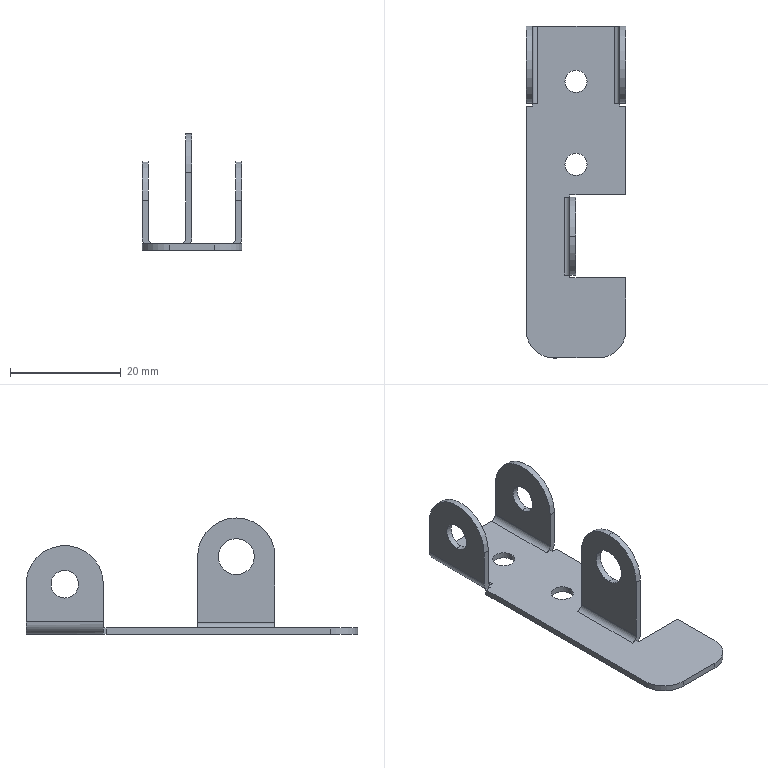Part | SolidWorks | features BaseBody 1 | 1 solid | 51 faces | box 18 x 60 x 21 mm | volume 1579 mm3 | plane 29 | cylinder 22 | commonest cylinder face diameters 4 x4 5 x4 14 x4 2 x3 4.4 x3 6.5 x2